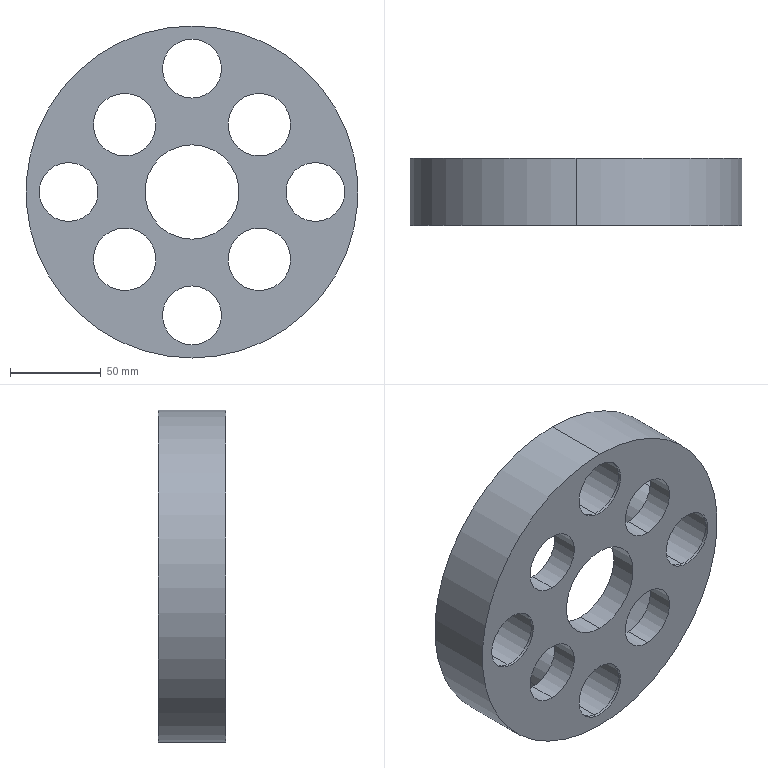Part | SolidWorks | features BaseBody 1 | 1 solid | 54 faces | box 183 x 37 x 183 mm | volume 386239 mm3 | cylinder 47 | plane 7 | commonest cylinder face diameters 20 x10 32.5 x8 34.5 x8 37 x8 46 x5 167 x4